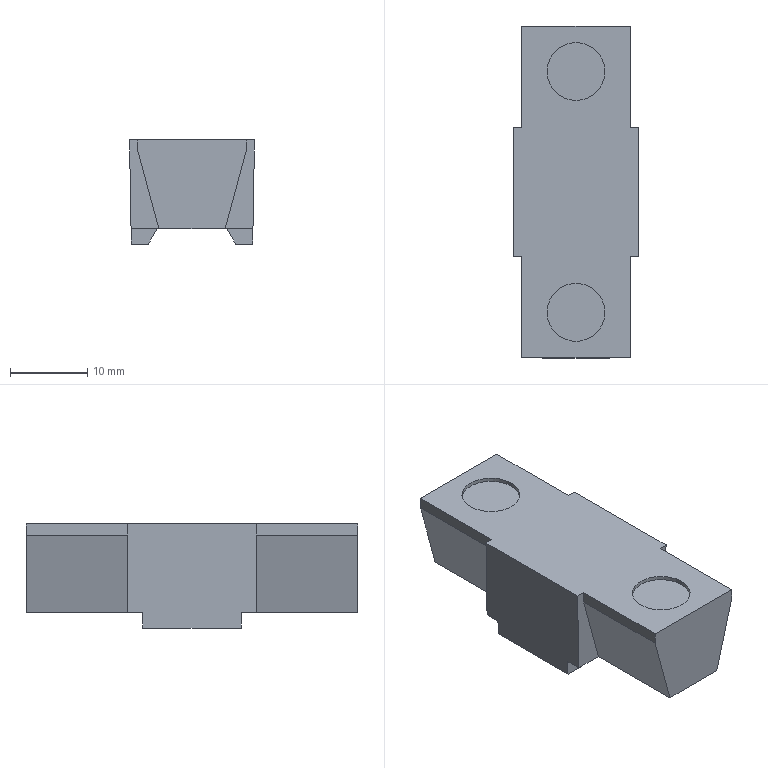Part | SolidWorks | features BaseBody 1 | 1 solid | 32 faces | box 16.2 x 43 x 13.5 mm | volume 6701 mm3 | plane 28 | cylinder 4 | commonest cylinder face diameters 7.5 x4
STEP:
#1=CARTESIAN_POINT('',(-3.75,15.6,26.));
#2=VERTEX_POINT('',#1);
#3=CARTESIAN_POINT('',(3.75,15.6,26.));
#4=VERTEX_POINT('',#3);
#5=CARTESIAN_POINT('',(0.,15.6,26.));
#6=DIRECTION('',(0.,0.,1.));
#7=DIRECTION('',(1.,0.,0.));
#8=AXIS2_PLACEMENT_3D('',#5,#6,#7);
#9=CIRCLE('',#8,3.75);
#10=EDGE_CURVE('',#2,#4,#9,.T.);
#11=ORIENTED_EDGE('',*,*,#10,.F.);
#12=CARTESIAN_POINT('',(-3.75,15.6,26.5));
#13=VERTEX_POINT('',#12);
#14=CARTESIAN_POINT('',(-3.75,15.6,26.));
#15=DIRECTION('',(0.,0.,1.));
#16=VECTOR('',#15,1000.);
#17=LINE('',#14,#16);
#18=EDGE_CURVE('',#2,#13,#17,.T.);
#19=ORIENTED_EDGE('',*,*,#18,.T.);
#20=CARTESIAN_POINT('',(3.75,15.6,26.5));
#21=VERTEX_POINT('',#20);
#22=CARTESIAN_POINT('',(0.,15.6,26.5));
#23=DIRECTION('',(0.,0.,1.));
#24=DIRECTION('',(1.,0.,0.));
#25=AXIS2_PLACEMENT_3D('',#22,#23,#24);
#26=CIRCLE('',#25,3.75);
#27=EDGE_CURVE('',#13,#21,#26,.T.);
#28=ORIENTED_EDGE('',*,*,#27,.T.);
#29=CARTESIAN_POINT('',(3.75,15.6,26.));
#30=DIRECTION('',(0.,0.,1.));
#31=VECTOR('',#30,1000.);
#32=LINE('',#29,#31);
#33=EDGE_CURVE('',#4,#21,#32,.T.);
#34=ORIENTED_EDGE('',*,*,#33,.F.);
#35=EDGE_LOOP('',(#11,#19,#28,#34));
#36=FACE_OUTER_BOUND('',#35,.T.);
#37=CARTESIAN_POINT('',(0.,15.6,26.));
#38=DIRECTION('',(0.,0.,1.));
#39=DIRECTION('',(1.,0.,0.));
#40=AXIS2_PLACEMENT_3D('',#37,#38,#39);
#41=CYLINDRICAL_SURFACE('',#40,3.75);
#42=ADVANCED_FACE('',(#36),#41,.F.);
#43=CARTESIAN_POINT('',(-3.75,-15.6,26.));
#44=VERTEX_POINT('',#43);
#45=CARTESIAN_POINT('',(3.75,-15.6,26.));
#46=VERTEX_POINT('',#45);
#47=CARTESIAN_POINT('',(0.,-15.6,26.));
#48=DIRECTION('',(0.,0.,1.));
#49=DIRECTION('',(1.,0.,0.));
#50=AXIS2_PLACEMENT_3D('',#47,#48,#49);
#51=CIRCLE('',#50,3.75);
#52=EDGE_CURVE('',#44,#46,#51,.T.);
#53=ORIENTED_EDGE('',*,*,#52,.F.);
#54=CARTESIAN_POINT('',(-3.75,-15.6,26.5));
#55=VERTEX_POINT('',#54);
#56=CARTESIAN_POINT('',(-3.75,-15.6,26.));
#57=DIRECTION('',(0.,0.,1.));
#58=VECTOR('',#57,1000.);
#59=LINE('',#56,#58);
#60=EDGE_CURVE('',#44,#55,#59,.T.);
#61=ORIENTED_EDGE('',*,*,#60,.T.);
#62=CARTESIAN_POINT('',(3.75,-15.6,26.5));
#63=VERTEX_POINT('',#62);
#64=CARTESIAN_POINT('',(0.,-15.6,26.5));
#65=DIRECTION('',(0.,0.,1.));
#66=DIRECTION('',(1.,0.,0.));
#67=AXIS2_PLACEMENT_3D('',#64,#65,#66);
#68=CIRCLE('',#67,3.75);
#69=EDGE_CURVE('',#55,#63,#68,.T.);
#70=ORIENTED_EDGE('',*,*,#69,.T.);
#71=CARTESIAN_POINT('',(3.75,-15.6,26.));
#72=DIRECTION('',(0.,0.,1.));
#73=VECTOR('',#72,1000.);
#74=LINE('',#71,#73);
#75=EDGE_CURVE('',#46,#63,#74,.T.);
#76=ORIENTED_EDGE('',*,*,#75,.F.);
#77=EDGE_LOOP('',(#53,#61,#70,#76));
#78=FACE_OUTER_BOUND('',#77,.T.);
#79=CARTESIAN_POINT('',(0.,-15.6,26.));
#80=DIRECTION('',(0.,0.,1.));
#81=DIRECTION('',(1.,0.,0.));
#82=AXIS2_PLACEMENT_3D('',#79,#80,#81);
#83=CYLINDRICAL_SURFACE('',#82,3.75);
#84=ADVANCED_FACE('',(#78),#83,.F.);
#85=CARTESIAN_POINT('',(7.864,6.4,13.));
#86=VERTEX_POINT('',#85);
#87=CARTESIAN_POINT('',(5.655,6.4,13.));
#88=VERTEX_POINT('',#87);
#89=CARTESIAN_POINT('',(7.864,6.4,13.));
#90=DIRECTION('',(-1.,0.,0.));
#91=VECTOR('',#90,1000.);
#92=LINE('',#89,#91);
#93=EDGE_CURVE('',#86,#88,#92,.T.);
#94=ORIENTED_EDGE('',*,*,#93,.F.);
#95=CARTESIAN_POINT('',(7.864,-6.4,13.));
#96=VERTEX_POINT('',#95);
#97=CARTESIAN_POINT('',(7.864,6.4,13.));
#98=DIRECTION('',(0.,-1.,0.));
#99=VECTOR('',#98,1000.);
#100=LINE('',#97,#99);
#101=EDGE_CURVE('',#86,#96,#100,.T.);
#102=ORIENTED_EDGE('',*,*,#101,.T.);
#103=CARTESIAN_POINT('',(5.655,-6.4,13.));
#104=VERTEX_POINT('',#103);
#105=CARTESIAN_POINT('',(7.864,-6.4,13.));
#106=DIRECTION('',(-1.,0.,0.));
#107=VECTOR('',#106,1000.);
#108=LINE('',#105,#107);
#109=EDGE_CURVE('',#96,#104,#108,.T.);
#110=ORIENTED_EDGE('',*,*,#109,.T.);
#111=CARTESIAN_POINT('',(5.655,6.4,13.));
#112=DIRECTION('',(0.,-1.,0.));
#113=VECTOR('',#112,1000.);
#114=LINE('',#111,#113);
#115=EDGE_CURVE('',#88,#104,#114,.T.);
#116=ORIENTED_EDGE('',*,*,#115,.F.);
#117=EDGE_LOOP('',(#94,#102,#110,#116));
#118=FACE_OUTER_BOUND('',#117,.T.);
#119=CARTESIAN_POINT('',(8.1,8.4,13.));
#120=DIRECTION('',(0.,0.,1.));
#121=DIRECTION('',(1.,0.,0.));
#122=AXIS2_PLACEMENT_3D('',#119,#120,#121);
#123=PLANE('',#122);
#124=ADVANCED_FACE('',(#118),#123,.F.);
#125=CARTESIAN_POINT('',(4.5,6.4,15.));
#126=VERTEX_POINT('',#125);
#127=CARTESIAN_POINT('',(5.655,6.4,13.));
#128=DIRECTION('',(-0.5,0.,0.866));
#129=VECTOR('',#128,1000.);
#130=LINE('',#127,#129);
#131=EDGE_CURVE('',#88,#126,#130,.T.);
#132=ORIENTED_EDGE('',*,*,#131,.T.);
#133=CARTESIAN_POINT('',(7.899,6.4,15.));
#134=VERTEX_POINT('',#133);
#135=CARTESIAN_POINT('',(7.899,6.4,15.));
#136=DIRECTION('',(-1.,0.,0.));
#137=VECTOR('',#136,1000.);
#138=LINE('',#135,#137);
#139=EDGE_CURVE('',#134,#126,#138,.T.);
#140=ORIENTED_EDGE('',*,*,#139,.F.);
#141=CARTESIAN_POINT('',(7.864,6.4,13.));
#142=DIRECTION('',(0.01745,0.,0.9998));
#143=VECTOR('',#142,1000.);
#144=LINE('',#141,#143);
#145=EDGE_CURVE('',#86,#134,#144,.T.);
#146=ORIENTED_EDGE('',*,*,#145,.F.);
#147=ORIENTED_EDGE('',*,*,#93,.T.);
#148=EDGE_LOOP('',(#132,#140,#146,#147));
#149=FACE_OUTER_BOUND('',#148,.T.);
#150=CARTESIAN_POINT('',(8.1,6.4,15.));
#151=DIRECTION('',(0.,1.,0.));
#152=DIRECTION('',(0.,0.,1.));
#153=AXIS2_PLACEMENT_3D('',#150,#151,#152);
#154=PLANE('',#153);
#155=ADVANCED_FACE('',(#149),#154,.T.);
#156=ORIENTED_EDGE('',*,*,#145,.T.);
#157=CARTESIAN_POINT('',(7.899,8.4,15.));
#158=VERTEX_POINT('',#157);
#159=CARTESIAN_POINT('',(7.899,6.4,15.));
#160=DIRECTION('',(0.,1.,0.));
#161=VECTOR('',#160,1000.);
#162=LINE('',#159,#161);
#163=EDGE_CURVE('',#134,#158,#162,.T.);
#164=ORIENTED_EDGE('',*,*,#163,.T.);
#165=CARTESIAN_POINT('',(8.1,8.4,26.5));
#166=VERTEX_POINT('',#165);
#167=CARTESIAN_POINT('',(8.1,8.4,26.5));
#168=DIRECTION('',(-0.01745,0.,-0.9998));
#169=VECTOR('',#168,1000.);
#170=LINE('',#167,#169);
#171=EDGE_CURVE('',#166,#158,#170,.T.);
#172=ORIENTED_EDGE('',*,*,#171,.F.);
#173=CARTESIAN_POINT('',(8.1,-8.4,26.5));
#174=VERTEX_POINT('',#173);
#175=CARTESIAN_POINT('',(8.1,8.4,26.5));
#176=DIRECTION('',(0.,-1.,0.));
#177=VECTOR('',#176,1000.);
#178=LINE('',#175,#177);
#179=EDGE_CURVE('',#166,#174,#178,.T.);
#180=ORIENTED_EDGE('',*,*,#179,.T.);
#181=CARTESIAN_POINT('',(7.899,-8.4,15.));
#182=VERTEX_POINT('',#181);
#183=CARTESIAN_POINT('',(8.1,-8.4,26.5));
#184=DIRECTION('',(-0.01745,0.,-0.9998));
#185=VECTOR('',#184,1000.);
#186=LINE('',#183,#185);
#187=EDGE_CURVE('',#174,#182,#186,.T.);
#188=ORIENTED_EDGE('',*,*,#187,.T.);
#189=CARTESIAN_POINT('',(7.899,-6.4,15.));
#190=VERTEX_POINT('',#189);
#191=CARTESIAN_POINT('',(7.899,-8.4,15.));
#192=DIRECTION('',(0.,1.,0.));
#193=VECTOR('',#192,1000.);
#194=LINE('',#191,#193);
#195=EDGE_CURVE('',#182,#190,#194,.T.);
#196=ORIENTED_EDGE('',*,*,#195,.T.);
#197=CARTESIAN_POINT('',(7.899,-6.4,15.));
#198=DIRECTION('',(-0.01745,0.,-0.9998));
#199=VECTOR('',#198,1000.);
#200=LINE('',#197,#199);
#201=EDGE_CURVE('',#190,#96,#200,.T.);
#202=ORIENTED_EDGE('',*,*,#201,.T.);
#203=ORIENTED_EDGE('',*,*,#101,.F.);
#204=EDGE_LOOP('',(#156,#164,#172,#180,#188,#196,#202,#203));
#205=FACE_OUTER_BOUND('',#204,.T.);
#206=CARTESIAN_POINT('',(7.864,21.5,13.));
#207=DIRECTION('',(0.9998,0.,-0.01745));
#208=DIRECTION('',(-0.01745,0.,-0.9998));
#209=AXIS2_PLACEMENT_3D('',#206,#207,#208);
#210=PLANE('',#209);
#211=ADVANCED_FACE('',(#205),#210,.T.);
#212=CARTESIAN_POINT('',(4.5,-6.4,15.));
#213=VERTEX_POINT('',#212);
#214=CARTESIAN_POINT('',(4.5,-6.4,15.));
#215=DIRECTION('',(0.5,0.,-0.866));
#216=VECTOR('',#215,1000.);
#217=LINE('',#214,#216);
#218=EDGE_CURVE('',#213,#104,#217,.T.);
#219=ORIENTED_EDGE('',*,*,#218,.T.);
#220=ORIENTED_EDGE('',*,*,#109,.F.);
#221=ORIENTED_EDGE('',*,*,#201,.F.);
#222=CARTESIAN_POINT('',(7.899,-6.4,15.));
#223=DIRECTION('',(-1.,0.,0.));
#224=VECTOR('',#223,1000.);
#225=LINE('',#222,#224);
#226=EDGE_CURVE('',#190,#213,#225,.T.);
#227=ORIENTED_EDGE('',*,*,#226,.T.);
#228=EDGE_LOOP('',(#219,#220,#221,#227));
#229=FACE_OUTER_BOUND('',#228,.T.);
#230=CARTESIAN_POINT('',(8.1,-6.4,13.));
#231=DIRECTION('',(0.,-1.,0.));
#232=DIRECTION('',(0.,0.,-1.));
#233=AXIS2_PLACEMENT_3D('',#230,#231,#232);
#234=PLANE('',#233);
#235=ADVANCED_FACE('',(#229),#234,.T.);
#236=ORIENTED_EDGE('',*,*,#131,.F.);
#237=ORIENTED_EDGE('',*,*,#115,.T.);
#238=ORIENTED_EDGE('',*,*,#218,.F.);
#239=CARTESIAN_POINT('',(4.5,6.4,15.));
#240=DIRECTION('',(0.,-1.,0.));
#241=VECTOR('',#240,1000.);
#242=LINE('',#239,#241);
#243=EDGE_CURVE('',#126,#213,#242,.T.);
#244=ORIENTED_EDGE('',*,*,#243,.F.);
#245=EDGE_LOOP('',(#236,#237,#238,#244));
#246=FACE_OUTER_BOUND('',#245,.T.);
#247=CARTESIAN_POINT('',(5.655,8.4,13.));
#248=DIRECTION('',(0.866,0.,0.5));
#249=DIRECTION('',(0.5,0.,-0.866));
#250=AXIS2_PLACEMENT_3D('',#247,#248,#249);
#251=PLANE('',#250);
#252=ADVANCED_FACE('',(#246),#251,.F.);
#253=CARTESIAN_POINT('',(-4.3,-8.4,15.));
#254=VERTEX_POINT('',#253);
#255=CARTESIAN_POINT('',(-7.899,-8.4,15.));
#256=VERTEX_POINT('',#255);
#257=CARTESIAN_POINT('',(-4.3,-8.4,15.));
#258=DIRECTION('',(-1.,0.,0.));
#259=VECTOR('',#258,1000.);
#260=LINE('',#257,#259);
#261=EDGE_CURVE('',#254,#256,#260,.T.);
#262=ORIENTED_EDGE('',*,*,#261,.T.);
#263=CARTESIAN_POINT('',(-7.899,-6.4,15.));
#264=VERTEX_POINT('',#263);
#265=CARTESIAN_POINT('',(-7.899,-6.4,15.));
#266=DIRECTION('',(0.,-1.,0.));
#267=VECTOR('',#266,1000.);
#268=LINE('',#265,#267);
#269=EDGE_CURVE('',#264,#256,#268,.T.);
#270=ORIENTED_EDGE('',*,*,#269,.F.);
#271=CARTESIAN_POINT('',(-4.5,-6.4,15.));
#272=VERTEX_POINT('',#271);
#273=CARTESIAN_POINT('',(-4.5,-6.4,15.));
#274=DIRECTION('',(-1.,0.,0.));
#275=VECTOR('',#274,1000.);
#276=LINE('',#273,#275);
#277=EDGE_CURVE('',#272,#264,#276,.T.);
#278=ORIENTED_EDGE('',*,*,#277,.F.);
#279=CARTESIAN_POINT('',(-4.5,6.4,15.));
#280=VERTEX_POINT('',#279);
#281=CARTESIAN_POINT('',(-4.5,6.4,15.));
#282=DIRECTION('',(0.,-1.,0.));
#283=VECTOR('',#282,1000.);
#284=LINE('',#281,#283);
#285=EDGE_CURVE('',#280,#272,#284,.T.);
#286=ORIENTED_EDGE('',*,*,#285,.F.);
#287=CARTESIAN_POINT('',(-7.899,6.4,15.));
#288=VERTEX_POINT('',#287);
#289=CARTESIAN_POINT('',(-4.5,6.4,15.));
#290=DIRECTION('',(-1.,0.,0.));
#291=VECTOR('',#290,1000.);
#292=LINE('',#289,#291);
#293=EDGE_CURVE('',#280,#288,#292,.T.);
#294=ORIENTED_EDGE('',*,*,#293,.T.);
#295=CARTESIAN_POINT('',(-7.899,8.4,15.));
#296=VERTEX_POINT('',#295);
#297=CARTESIAN_POINT('',(-7.899,8.4,15.));
#298=DIRECTION('',(0.,-1.,0.));
#299=VECTOR('',#298,1000.);
#300=LINE('',#297,#299);
#301=EDGE_CURVE('',#296,#288,#300,.T.);
#302=ORIENTED_EDGE('',*,*,#301,.F.);
#303=CARTESIAN_POINT('',(-4.3,8.4,15.));
#304=VERTEX_POINT('',#303);
#305=CARTESIAN_POINT('',(-4.3,8.4,15.));
#306=DIRECTION('',(-1.,0.,0.));
#307=VECTOR('',#306,1000.);
#308=LINE('',#305,#307);
#309=EDGE_CURVE('',#304,#296,#308,.T.);
#310=ORIENTED_EDGE('',*,*,#309,.F.);
#311=CARTESIAN_POINT('',(-4.3,21.5,15.));
#312=VERTEX_POINT('',#311);
#313=CARTESIAN_POINT('',(-4.3,21.5,15.));
#314=DIRECTION('',(0.,-1.,0.));
#315=VECTOR('',#314,1000.);
#316=LINE('',#313,#315);
#317=EDGE_CURVE('',#312,#304,#316,.T.);
#318=ORIENTED_EDGE('',*,*,#317,.F.);
#319=CARTESIAN_POINT('',(4.3,21.5,15.));
#320=VERTEX_POINT('',#319);
#321=CARTESIAN_POINT('',(4.3,21.5,15.));
#322=DIRECTION('',(-1.,0.,0.));
#323=VECTOR('',#322,1000.);
#324=LINE('',#321,#323);
#325=EDGE_CURVE('',#320,#312,#324,.T.);
#326=ORIENTED_EDGE('',*,*,#325,.F.);
#327=CARTESIAN_POINT('',(4.3,8.4,15.));
#328=VERTEX_POINT('',#327);
#329=CARTESIAN_POINT('',(4.3,21.5,15.));
#330=DIRECTION('',(0.,-1.,0.));
#331=VECTOR('',#330,1000.);
#332=LINE('',#329,#331);
#333=EDGE_CURVE('',#320,#328,#332,.T.);
#334=ORIENTED_EDGE('',*,*,#333,.T.);
#335=CARTESIAN_POINT('',(7.899,8.4,15.));
#336=DIRECTION('',(-1.,0.,0.));
#337=VECTOR('',#336,1000.);
#338=LINE('',#335,#337);
#339=EDGE_CURVE('',#158,#328,#338,.T.);
#340=ORIENTED_EDGE('',*,*,#339,.F.);
#341=ORIENTED_EDGE('',*,*,#163,.F.);
#342=ORIENTED_EDGE('',*,*,#139,.T.);
#343=ORIENTED_EDGE('',*,*,#243,.T.);
#344=ORIENTED_EDGE('',*,*,#226,.F.);
#345=ORIENTED_EDGE('',*,*,#195,.F.);
#346=CARTESIAN_POINT('',(4.3,-8.4,15.));
#347=VERTEX_POINT('',#346);
#348=CARTESIAN_POINT('',(7.899,-8.4,15.));
#349=DIRECTION('',(-1.,0.,0.));
#350=VECTOR('',#349,1000.);
#351=LINE('',#348,#350);
#352=EDGE_CURVE('',#182,#347,#351,.T.);
#353=ORIENTED_EDGE('',*,*,#352,.T.);
#354=CARTESIAN_POINT('',(4.3,-21.5,15.));
#355=VERTEX_POINT('',#354);
#356=CARTESIAN_POINT('',(4.3,-8.4,15.));
#357=DIRECTION('',(0.,-1.,0.));
#358=VECTOR('',#357,1000.);
#359=LINE('',#356,#358);
#360=EDGE_CURVE('',#347,#355,#359,.T.);
#361=ORIENTED_EDGE('',*,*,#360,.T.);
#362=CARTESIAN_POINT('',(-4.3,-21.5,15.));
#363=VERTEX_POINT('',#362);
#364=CARTESIAN_POINT('',(4.3,-21.5,15.));
#365=DIRECTION('',(-1.,0.,0.));
#366=VECTOR('',#365,1000.);
#367=LINE('',#364,#366);
#368=EDGE_CURVE('',#355,#363,#367,.T.);
#369=ORIENTED_EDGE('',*,*,#368,.T.);
#370=CARTESIAN_POINT('',(-4.3,-8.4,15.));
#371=DIRECTION('',(0.,-1.,0.));
#372=VECTOR('',#371,1000.);
#373=LINE('',#370,#372);
#374=EDGE_CURVE('',#254,#363,#373,.T.);
#375=ORIENTED_EDGE('',*,*,#374,.F.);
#376=EDGE_LOOP('',(#262,#270,#278,#286,#294,#302,#310,#318,#326,#334,#340,#341,#342,#343,#344,#345,#353,#361,#369,#375));
#377=FACE_OUTER_BOUND('',#376,.T.);
#378=CARTESIAN_POINT('',(4.3,21.5,15.));
#379=DIRECTION('',(0.,0.,1.));
#380=DIRECTION('',(1.,0.,0.));
#381=AXIS2_PLACEMENT_3D('',#378,#379,#380);
#382=PLANE('',#381);
#383=ADVANCED_FACE('',(#377),#382,.F.);
#384=ORIENTED_EDGE('',*,*,#171,.T.);
#385=ORIENTED_EDGE('',*,*,#339,.T.);
#386=CARTESIAN_POINT('',(7.,8.4,25.));
#387=VERTEX_POINT('',#386);
#388=CARTESIAN_POINT('',(7.,8.4,25.));
#389=DIRECTION('',(-0.2607,0.,-0.9654));
#390=VECTOR('',#389,1000.);
#391=LINE('',#388,#390);
#392=EDGE_CURVE('',#387,#328,#391,.T.);
#393=ORIENTED_EDGE('',*,*,#392,.F.);
#394=CARTESIAN_POINT('',(7.,8.4,26.5));
#395=VERTEX_POINT('',#394);
#396=CARTESIAN_POINT('',(7.,8.4,26.5));
#397=DIRECTION('',(0.,0.,-1.));
#398=VECTOR('',#397,1000.);
#399=LINE('',#396,#398);
#400=EDGE_CURVE('',#395,#387,#399,.T.);
#401=ORIENTED_EDGE('',*,*,#400,.F.);
#402=CARTESIAN_POINT('',(7.,8.4,26.5));
#403=DIRECTION('',(1.,0.,0.));
#404=VECTOR('',#403,1000.);
#405=LINE('',#402,#404);
#406=EDGE_CURVE('',#395,#166,#405,.T.);
#407=ORIENTED_EDGE('',*,*,#406,.T.);
#408=EDGE_LOOP('',(#384,#385,#393,#401,#407));
#409=FACE_OUTER_BOUND('',#408,.T.);
#410=CARTESIAN_POINT('',(0.,8.4,0.));
#411=DIRECTION('',(0.,1.,0.));
#412=DIRECTION('',(0.,0.,1.));
#413=AXIS2_PLACEMENT_3D('',#410,#411,#412);
#414=PLANE('',#413);
#415=ADVANCED_FACE('',(#409),#414,.T.);
#416=CARTESIAN_POINT('',(0.,-15.6,26.5));
#417=DIRECTION('',(0.,0.,1.));
#418=DIRECTION('',(1.,0.,0.));
#419=AXIS2_PLACEMENT_3D('',#416,#417,#418);
#420=CIRCLE('',#419,3.75);
#421=EDGE_CURVE('',#63,#55,#420,.T.);
#422=ORIENTED_EDGE('',*,*,#421,.F.);
#423=ORIENTED_EDGE('',*,*,#69,.F.);
#424=EDGE_LOOP('',(#422,#423));
#425=FACE_BOUND('',#424,.T.);
#426=CARTESIAN_POINT('',(0.,15.6,26.5));
#427=DIRECTION('',(0.,0.,1.));
#428=DIRECTION('',(1.,0.,0.));
#429=AXIS2_PLACEMENT_3D('',#426,#427,#428);
#430=CIRCLE('',#429,3.75);
#431=EDGE_CURVE('',#21,#13,#430,.T.);
#432=ORIENTED_EDGE('',*,*,#431,.F.);
#433=ORIENTED_EDGE('',*,*,#27,.F.);
#434=EDGE_LOOP('',(#432,#433));
#435=FACE_BOUND('',#434,.T.);
#436=CARTESIAN_POINT('',(-7.,21.5,26.5));
#437=VERTEX_POINT('',#436);
#438=CARTESIAN_POINT('',(-7.,8.4,26.5));
#439=VERTEX_POINT('',#438);
#440=CARTESIAN_POINT('',(-7.,21.5,26.5));
#441=DIRECTION('',(0.,-1.,0.));
#442=VECTOR('',#441,1000.);
#443=LINE('',#440,#442);
#444=EDGE_CURVE('',#437,#439,#443,.T.);
#445=ORIENTED_EDGE('',*,*,#444,.T.);
#446=CARTESIAN_POINT('',(-8.1,8.4,26.5));
#447=VERTEX_POINT('',#446);
#448=CARTESIAN_POINT('',(-8.1,8.4,26.5));
#449=DIRECTION('',(1.,0.,0.));
#450=VECTOR('',#449,1000.);
#451=LINE('',#448,#450);
#452=EDGE_CURVE('',#447,#439,#451,.T.);
#453=ORIENTED_EDGE('',*,*,#452,.F.);
#454=CARTESIAN_POINT('',(-8.1,-8.4,26.5));
#455=VERTEX_POINT('',#454);
#456=CARTESIAN_POINT('',(-8.1,8.4,26.5));
#457=DIRECTION('',(0.,-1.,0.));
#458=VECTOR('',#457,1000.);
#459=LINE('',#456,#458);
#460=EDGE_CURVE('',#447,#455,#459,.T.);
#461=ORIENTED_EDGE('',*,*,#460,.T.);
#462=CARTESIAN_POINT('',(-7.,-8.4,26.5));
#463=VERTEX_POINT('',#462);
#464=CARTESIAN_POINT('',(-8.1,-8.4,26.5));
#465=DIRECTION('',(1.,0.,0.));
#466=VECTOR('',#465,1000.);
#467=LINE('',#464,#466);
#468=EDGE_CURVE('',#455,#463,#467,.T.);
#469=ORIENTED_EDGE('',*,*,#468,.T.);
#470=CARTESIAN_POINT('',(-7.,-21.5,26.5));
#471=VERTEX_POINT('',#470);
#472=CARTESIAN_POINT('',(-7.,-8.4,26.5));
#473=DIRECTION('',(0.,-1.,0.));
#474=VECTOR('',#473,1000.);
#475=LINE('',#472,#474);
#476=EDGE_CURVE('',#463,#471,#475,.T.);
#477=ORIENTED_EDGE('',*,*,#476,.T.);
#478=CARTESIAN_POINT('',(7.,-21.5,26.5));
#479=VERTEX_POINT('',#478);
#480=CARTESIAN_POINT('',(-7.,-21.5,26.5));
#481=DIRECTION('',(1.,0.,0.));
#482=VECTOR('',#481,1000.);
#483=LINE('',#480,#482);
#484=EDGE_CURVE('',#471,#479,#483,.T.);
#485=ORIENTED_EDGE('',*,*,#484,.T.);
#486=CARTESIAN_POINT('',(7.,-8.4,26.5));
#487=VERTEX_POINT('',#486);
#488=CARTESIAN_POINT('',(7.,-8.4,26.5));
#489=DIRECTION('',(0.,-1.,0.));
#490=VECTOR('',#489,1000.);
#491=LINE('',#488,#490);
#492=EDGE_CURVE('',#487,#479,#491,.T.);
#493=ORIENTED_EDGE('',*,*,#492,.F.);
#494=CARTESIAN_POINT('',(7.,-8.4,26.5));
#495=DIRECTION('',(1.,0.,0.));
#496=VECTOR('',#495,1000.);
#497=LINE('',#494,#496);
#498=EDGE_CURVE('',#487,#174,#497,.T.);
#499=ORIENTED_EDGE('',*,*,#498,.T.);
#500=ORIENTED_EDGE('',*,*,#179,.F.);
#501=ORIENTED_EDGE('',*,*,#406,.F.);
#502=CARTESIAN_POINT('',(7.,21.5,26.5));
#503=VERTEX_POINT('',#502);
#504=CARTESIAN_POINT('',(7.,21.5,26.5));
#505=DIRECTION('',(0.,-1.,0.));
#506=VECTOR('',#505,1000.);
#507=LINE('',#504,#506);
#508=EDGE_CURVE('',#503,#395,#507,.T.);
#509=ORIENTED_EDGE('',*,*,#508,.F.);
#510=CARTESIAN_POINT('',(-7.,21.5,26.5));
#511=DIRECTION('',(1.,0.,0.));
#512=VECTOR('',#511,1000.);
#513=LINE('',#510,#512);
#514=EDGE_CURVE('',#437,#503,#513,.T.);
#515=ORIENTED_EDGE('',*,*,#514,.F.);
#516=EDGE_LOOP('',(#445,#453,#461,#469,#477,#485,#493,#499,#500,#501,#509,#515));
#517=FACE_OUTER_BOUND('',#516,.T.);
#518=CARTESIAN_POINT('',(-7.,21.5,26.5));
#519=DIRECTION('',(0.,0.,-1.));
#520=DIRECTION('',(-1.,0.,0.));
#521=AXIS2_PLACEMENT_3D('',#518,#519,#520);
#522=PLANE('',#521);
#523=ADVANCED_FACE('',(#425,#435,#517),#522,.F.);
#524=ORIENTED_EDGE('',*,*,#352,.F.);
#525=ORIENTED_EDGE('',*,*,#187,.F.);
#526=ORIENTED_EDGE('',*,*,#498,.F.);
#527=CARTESIAN_POINT('',(7.,-8.4,25.));
#528=VERTEX_POINT('',#527);
#529=CARTESIAN_POINT('',(7.,-8.4,26.5));
#530=DIRECTION('',(0.,0.,-1.));
#531=VECTOR('',#530,1000.);
#532=LINE('',#529,#531);
#533=EDGE_CURVE('',#487,#528,#532,.T.);
#534=ORIENTED_EDGE('',*,*,#533,.T.);
#535=CARTESIAN_POINT('',(7.,-8.4,25.));
#536=DIRECTION('',(-0.2607,0.,-0.9654));
#537=VECTOR('',#536,1000.);
#538=LINE('',#535,#537);
#539=EDGE_CURVE('',#528,#347,#538,.T.);
#540=ORIENTED_EDGE('',*,*,#539,.T.);
#541=EDGE_LOOP('',(#524,#525,#526,#534,#540));
#542=FACE_OUTER_BOUND('',#541,.T.);
#543=CARTESIAN_POINT('',(0.,-8.4,0.));
#544=DIRECTION('',(0.,1.,0.));
#545=DIRECTION('',(0.,0.,1.));
#546=AXIS2_PLACEMENT_3D('',#543,#544,#545);
#547=PLANE('',#546);
#548=ADVANCED_FACE('',(#542),#547,.F.);
#549=CARTESIAN_POINT('',(-7.899,-8.4,15.));
#550=DIRECTION('',(-0.01745,0.,0.9998));
#551=VECTOR('',#550,1000.);
#552=LINE('',#549,#551);
#553=EDGE_CURVE('',#256,#455,#552,.T.);
#554=ORIENTED_EDGE('',*,*,#553,.F.);
#555=ORIENTED_EDGE('',*,*,#261,.F.);
#556=CARTESIAN_POINT('',(-7.,-8.4,25.));
#557=VERTEX_POINT('',#556);
#558=CARTESIAN_POINT('',(-4.3,-8.4,15.));
#559=DIRECTION('',(-0.2607,0.,0.9654));
#560=VECTOR('',#559,1000.);
#561=LINE('',#558,#560);
#562=EDGE_CURVE('',#254,#557,#561,.T.);
#563=ORIENTED_EDGE('',*,*,#562,.T.);
#564=CARTESIAN_POINT('',(-7.,-8.4,25.));
#565=DIRECTION('',(0.,0.,1.));
#566=VECTOR('',#565,1000.);
#567=LINE('',#564,#566);
#568=EDGE_CURVE('',#557,#463,#567,.T.);
#569=ORIENTED_EDGE('',*,*,#568,.T.);
#570=ORIENTED_EDGE('',*,*,#468,.F.);
#571=EDGE_LOOP('',(#554,#555,#563,#569,#570));
#572=FACE_OUTER_BOUND('',#571,.T.);
#573=CARTESIAN_POINT('',(0.,-8.4,0.));
#574=DIRECTION('',(0.,1.,0.));
#575=DIRECTION('',(0.,0.,1.));
#576=AXIS2_PLACEMENT_3D('',#573,#574,#575);
#577=PLANE('',#576);
#578=ADVANCED_FACE('',(#572),#577,.F.);
#579=CARTESIAN_POINT('',(-7.899,8.4,15.));
#580=DIRECTION('',(-0.01745,0.,0.9998));
#581=VECTOR('',#580,1000.);
#582=LINE('',#579,#581);
#583=EDGE_CURVE('',#296,#447,#582,.T.);
#584=ORIENTED_EDGE('',*,*,#583,.F.);
#585=ORIENTED_EDGE('',*,*,#301,.T.);
#586=CARTESIAN_POINT('',(-7.864,6.4,13.));
#587=VERTEX_POINT('',#586);
#588=CARTESIAN_POINT('',(-7.899,6.4,15.));
#589=DIRECTION('',(0.01745,0.,-0.9998));
#590=VECTOR('',#589,1000.);
#591=LINE('',#588,#590);
#592=EDGE_CURVE('',#288,#587,#591,.T.);
#593=ORIENTED_EDGE('',*,*,#592,.T.);
#594=CARTESIAN_POINT('',(-7.864,-6.4,13.));
#595=VERTEX_POINT('',#594);
#596=CARTESIAN_POINT('',(-7.864,6.4,13.));
#597=DIRECTION('',(0.,-1.,0.));
#598=VECTOR('',#597,1000.);
#599=LINE('',#596,#598);
#600=EDGE_CURVE('',#587,#595,#599,.T.);
#601=ORIENTED_EDGE('',*,*,#600,.T.);
#602=CARTESIAN_POINT('',(-7.864,-6.4,13.));
#603=DIRECTION('',(-0.01745,0.,0.9998));
#604=VECTOR('',#603,1000.);
#605=LINE('',#602,#604);
#606=EDGE_CURVE('',#595,#264,#605,.T.);
#607=ORIENTED_EDGE('',*,*,#606,.T.);
#608=ORIENTED_EDGE('',*,*,#269,.T.);
#609=ORIENTED_EDGE('',*,*,#553,.T.);
#610=ORIENTED_EDGE('',*,*,#460,.F.);
#611=EDGE_LOOP('',(#584,#585,#593,#601,#607,#608,#609,#610));
#612=FACE_OUTER_BOUND('',#611,.T.);
#613=CARTESIAN_POINT('',(-8.1,21.5,26.5));
#614=DIRECTION('',(-0.9998,0.,-0.01745));
#615=DIRECTION('',(-0.01745,0.,0.9998));
#616=AXIS2_PLACEMENT_3D('',#613,#614,#615);
#617=PLANE('',#616);
#618=ADVANCED_FACE('',(#612),#617,.T.);
#619=CARTESIAN_POINT('',(-5.655,-6.4,13.));
#620=VERTEX_POINT('',#619);
#621=CARTESIAN_POINT('',(-5.655,-6.4,13.));
#622=DIRECTION('',(0.5,0.,0.866));
#623=VECTOR('',#622,1000.);
#624=LINE('',#621,#623);
#625=EDGE_CURVE('',#620,#272,#624,.T.);
#626=ORIENTED_EDGE('',*,*,#625,.T.);
#627=ORIENTED_EDGE('',*,*,#277,.T.);
#628=ORIENTED_EDGE('',*,*,#606,.F.);
#629=CARTESIAN_POINT('',(-5.655,-6.4,13.));
#630=DIRECTION('',(-1.,0.,0.));
#631=VECTOR('',#630,1000.);
#632=LINE('',#629,#631);
#633=EDGE_CURVE('',#620,#595,#632,.T.);
#634=ORIENTED_EDGE('',*,*,#633,.F.);
#635=EDGE_LOOP('',(#626,#627,#628,#634));
#636=FACE_OUTER_BOUND('',#635,.T.);
#637=CARTESIAN_POINT('',(8.1,-6.4,13.));
#638=DIRECTION('',(0.,-1.,0.));
#639=DIRECTION('',(0.,0.,-1.));
#640=AXIS2_PLACEMENT_3D('',#637,#638,#639);
#641=PLANE('',#640);
#642=ADVANCED_FACE('',(#636),#641,.T.);
#643=CARTESIAN_POINT('',(-5.655,6.4,13.));
#644=VERTEX_POINT('',#643);
#645=CARTESIAN_POINT('',(-4.5,6.4,15.));
#646=DIRECTION('',(-0.5,0.,-0.866));
#647=VECTOR('',#646,1000.);
#648=LINE('',#645,#647);
#649=EDGE_CURVE('',#280,#644,#648,.T.);
#650=ORIENTED_EDGE('',*,*,#649,.F.);
#651=ORIENTED_EDGE('',*,*,#285,.T.);
#652=ORIENTED_EDGE('',*,*,#625,.F.);
#653=CARTESIAN_POINT('',(-5.655,6.4,13.));
#654=DIRECTION('',(0.,-1.,0.));
#655=VECTOR('',#654,1000.);
#656=LINE('',#653,#655);
#657=EDGE_CURVE('',#644,#620,#656,.T.);
#658=ORIENTED_EDGE('',*,*,#657,.F.);
#659=EDGE_LOOP('',(#650,#651,#652,#658));
#660=FACE_OUTER_BOUND('',#659,.T.);
#661=CARTESIAN_POINT('',(-4.5,8.4,15.));
#662=DIRECTION('',(-0.866,0.,0.5));
#663=DIRECTION('',(0.5,0.,0.866));
#664=AXIS2_PLACEMENT_3D('',#661,#662,#663);
#665=PLANE('',#664);
#666=ADVANCED_FACE('',(#660),#665,.F.);
#667=ORIENTED_EDGE('',*,*,#649,.T.);
#668=CARTESIAN_POINT('',(-5.655,6.4,13.));
#669=DIRECTION('',(-1.,0.,0.));
#670=VECTOR('',#669,1000.);
#671=LINE('',#668,#670);
#672=EDGE_CURVE('',#644,#587,#671,.T.);
#673=ORIENTED_EDGE('',*,*,#672,.T.);
#674=ORIENTED_EDGE('',*,*,#592,.F.);
#675=ORIENTED_EDGE('',*,*,#293,.F.);
#676=EDGE_LOOP('',(#667,#673,#674,#675));
#677=FACE_OUTER_BOUND('',#676,.T.);
#678=CARTESIAN_POINT('',(8.1,6.4,15.));
#679=DIRECTION('',(0.,1.,0.));
#680=DIRECTION('',(0.,0.,1.));
#681=AXIS2_PLACEMENT_3D('',#678,#679,#680);
#682=PLANE('',#681);
#683=ADVANCED_FACE('',(#677),#682,.T.);
#684=ORIENTED_EDGE('',*,*,#309,.T.);
#685=ORIENTED_EDGE('',*,*,#583,.T.);
#686=ORIENTED_EDGE('',*,*,#452,.T.);
#687=CARTESIAN_POINT('',(-7.,8.4,25.));
#688=VERTEX_POINT('',#687);
#689=CARTESIAN_POINT('',(-7.,8.4,25.));
#690=DIRECTION('',(0.,0.,1.));
#691=VECTOR('',#690,1000.);
#692=LINE('',#689,#691);
#693=EDGE_CURVE('',#688,#439,#692,.T.);
#694=ORIENTED_EDGE('',*,*,#693,.F.);
#695=CARTESIAN_POINT('',(-4.3,8.4,15.));
#696=DIRECTION('',(-0.2607,0.,0.9654));
#697=VECTOR('',#696,1000.);
#698=LINE('',#695,#697);
#699=EDGE_CURVE('',#304,#688,#698,.T.);
#700=ORIENTED_EDGE('',*,*,#699,.F.);
#701=EDGE_LOOP('',(#684,#685,#686,#694,#700));
#702=FACE_OUTER_BOUND('',#701,.T.);
#703=CARTESIAN_POINT('',(0.,8.4,0.));
#704=DIRECTION('',(0.,1.,0.));
#705=DIRECTION('',(0.,0.,1.));
#706=AXIS2_PLACEMENT_3D('',#703,#704,#705);
#707=PLANE('',#706);
#708=ADVANCED_FACE('',(#702),#707,.T.);
#709=ORIENTED_EDGE('',*,*,#317,.T.);
#710=ORIENTED_EDGE('',*,*,#699,.T.);
#711=CARTESIAN_POINT('',(-7.,21.5,25.));
#712=VERTEX_POINT('',#711);
#713=CARTESIAN_POINT('',(-7.,21.5,25.));
#714=DIRECTION('',(0.,-1.,0.));
#715=VECTOR('',#714,1000.);
#716=LINE('',#713,#715);
#717=EDGE_CURVE('',#712,#688,#716,.T.);
#718=ORIENTED_EDGE('',*,*,#717,.F.);
#719=CARTESIAN_POINT('',(-4.3,21.5,15.));
#720=DIRECTION('',(-0.2607,0.,0.9654));
#721=VECTOR('',#720,1000.);
#722=LINE('',#719,#721);
#723=EDGE_CURVE('',#312,#712,#722,.T.);
#724=ORIENTED_EDGE('',*,*,#723,.F.);
#725=EDGE_LOOP('',(#709,#710,#718,#724));
#726=FACE_OUTER_BOUND('',#725,.T.);
#727=CARTESIAN_POINT('',(-4.3,21.5,15.));
#728=DIRECTION('',(0.9654,0.,0.2607));
#729=DIRECTION('',(0.2607,0.,-0.9654));
#730=AXIS2_PLACEMENT_3D('',#727,#728,#729);
#731=PLANE('',#730);
#732=ADVANCED_FACE('',(#726),#731,.F.);
#733=ORIENTED_EDGE('',*,*,#723,.T.);
#734=CARTESIAN_POINT('',(-7.,21.5,25.));
#735=DIRECTION('',(0.,0.,1.));
#736=VECTOR('',#735,1000.);
#737=LINE('',#734,#736);
#738=EDGE_CURVE('',#712,#437,#737,.T.);
#739=ORIENTED_EDGE('',*,*,#738,.T.);
#740=ORIENTED_EDGE('',*,*,#514,.T.);
#741=CARTESIAN_POINT('',(7.,21.5,25.));
#742=VERTEX_POINT('',#741);
#743=CARTESIAN_POINT('',(7.,21.5,26.5));
#744=DIRECTION('',(0.,0.,-1.));
#745=VECTOR('',#744,1000.);
#746=LINE('',#743,#745);
#747=EDGE_CURVE('',#503,#742,#746,.T.);
#748=ORIENTED_EDGE('',*,*,#747,.T.);
#749=CARTESIAN_POINT('',(7.,21.5,25.));
#750=DIRECTION('',(-0.2607,0.,-0.9654));
#751=VECTOR('',#750,1000.);
#752=LINE('',#749,#751);
#753=EDGE_CURVE('',#742,#320,#752,.T.);
#754=ORIENTED_EDGE('',*,*,#753,.T.);
#755=ORIENTED_EDGE('',*,*,#325,.T.);
#756=EDGE_LOOP('',(#733,#739,#740,#748,#754,#755));
#757=FACE_OUTER_BOUND('',#756,.T.);
#758=CARTESIAN_POINT('',(0.,21.5,0.));
#759=DIRECTION('',(0.,1.,0.));
#760=DIRECTION('',(0.,0.,1.));
#761=AXIS2_PLACEMENT_3D('',#758,#759,#760);
#762=PLANE('',#761);
#763=ADVANCED_FACE('',(#757),#762,.T.);
#764=CARTESIAN_POINT('',(7.,21.5,25.));
#765=DIRECTION('',(0.,-1.,0.));
#766=VECTOR('',#765,1000.);
#767=LINE('',#764,#766);
#768=EDGE_CURVE('',#742,#387,#767,.T.);
#769=ORIENTED_EDGE('',*,*,#768,.T.);
#770=ORIENTED_EDGE('',*,*,#392,.T.);
#771=ORIENTED_EDGE('',*,*,#333,.F.);
#772=ORIENTED_EDGE('',*,*,#753,.F.);
#773=EDGE_LOOP('',(#769,#770,#771,#772));
#774=FACE_OUTER_BOUND('',#773,.T.);
#775=CARTESIAN_POINT('',(7.,21.5,25.));
#776=DIRECTION('',(-0.9654,0.,0.2607));
#777=DIRECTION('',(0.2607,0.,0.9654));
#778=AXIS2_PLACEMENT_3D('',#775,#776,#777);
#779=PLANE('',#778);
#780=ADVANCED_FACE('',(#774),#779,.F.);
#781=ORIENTED_EDGE('',*,*,#539,.F.);
#782=CARTESIAN_POINT('',(7.,-21.5,25.));
#783=VERTEX_POINT('',#782);
#784=CARTESIAN_POINT('',(7.,-8.4,25.));
#785=DIRECTION('',(0.,-1.,0.));
#786=VECTOR('',#785,1000.);
#787=LINE('',#784,#786);
#788=EDGE_CURVE('',#528,#783,#787,.T.);
#789=ORIENTED_EDGE('',*,*,#788,.T.);
#790=CARTESIAN_POINT('',(7.,-21.5,25.));
#791=DIRECTION('',(-0.2607,0.,-0.9654));
#792=VECTOR('',#791,1000.);
#793=LINE('',#790,#792);
#794=EDGE_CURVE('',#783,#355,#793,.T.);
#795=ORIENTED_EDGE('',*,*,#794,.T.);
#796=ORIENTED_EDGE('',*,*,#360,.F.);
#797=EDGE_LOOP('',(#781,#789,#795,#796));
#798=FACE_OUTER_BOUND('',#797,.T.);
#799=CARTESIAN_POINT('',(7.,21.5,25.));
#800=DIRECTION('',(-0.9654,0.,0.2607));
#801=DIRECTION('',(0.2607,0.,0.9654));
#802=AXIS2_PLACEMENT_3D('',#799,#800,#801);
#803=PLANE('',#802);
#804=ADVANCED_FACE('',(#798),#803,.F.);
#805=CARTESIAN_POINT('',(-7.,-21.5,25.));
#806=VERTEX_POINT('',#805);
#807=CARTESIAN_POINT('',(-4.3,-21.5,15.));
#808=DIRECTION('',(-0.2607,0.,0.9654));
#809=VECTOR('',#808,1000.);
#810=LINE('',#807,#809);
#811=EDGE_CURVE('',#363,#806,#810,.T.);
#812=ORIENTED_EDGE('',*,*,#811,.F.);
#813=ORIENTED_EDGE('',*,*,#368,.F.);
#814=ORIENTED_EDGE('',*,*,#794,.F.);
#815=CARTESIAN_POINT('',(7.,-21.5,26.5));
#816=DIRECTION('',(0.,0.,-1.));
#817=VECTOR('',#816,1000.);
#818=LINE('',#815,#817);
#819=EDGE_CURVE('',#479,#783,#818,.T.);
#820=ORIENTED_EDGE('',*,*,#819,.F.);
#821=ORIENTED_EDGE('',*,*,#484,.F.);
#822=CARTESIAN_POINT('',(-7.,-21.5,25.));
#823=DIRECTION('',(0.,0.,1.));
#824=VECTOR('',#823,1000.);
#825=LINE('',#822,#824);
#826=EDGE_CURVE('',#806,#471,#825,.T.);
#827=ORIENTED_EDGE('',*,*,#826,.F.);
#828=EDGE_LOOP('',(#812,#813,#814,#820,#821,#827));
#829=FACE_OUTER_BOUND('',#828,.T.);
#830=CARTESIAN_POINT('',(0.,-21.5,0.));
#831=DIRECTION('',(0.,1.,0.));
#832=DIRECTION('',(0.,0.,1.));
#833=AXIS2_PLACEMENT_3D('',#830,#831,#832);
#834=PLANE('',#833);
#835=ADVANCED_FACE('',(#829),#834,.F.);
#836=ORIENTED_EDGE('',*,*,#562,.F.);
#837=ORIENTED_EDGE('',*,*,#374,.T.);
#838=ORIENTED_EDGE('',*,*,#811,.T.);
#839=CARTESIAN_POINT('',(-7.,-8.4,25.));
#840=DIRECTION('',(0.,-1.,0.));
#841=VECTOR('',#840,1000.);
#842=LINE('',#839,#841);
#843=EDGE_CURVE('',#557,#806,#842,.T.);
#844=ORIENTED_EDGE('',*,*,#843,.F.);
#845=EDGE_LOOP('',(#836,#837,#838,#844));
#846=FACE_OUTER_BOUND('',#845,.T.);
#847=CARTESIAN_POINT('',(-4.3,21.5,15.));
#848=DIRECTION('',(0.9654,0.,0.2607));
#849=DIRECTION('',(0.2607,0.,-0.9654));
#850=AXIS2_PLACEMENT_3D('',#847,#848,#849);
#851=PLANE('',#850);
#852=ADVANCED_FACE('',(#846),#851,.F.);
#853=ORIENTED_EDGE('',*,*,#508,.T.);
#854=ORIENTED_EDGE('',*,*,#400,.T.);
#855=ORIENTED_EDGE('',*,*,#768,.F.);
#856=ORIENTED_EDGE('',*,*,#747,.F.);
#857=EDGE_LOOP('',(#853,#854,#855,#856));
#858=FACE_OUTER_BOUND('',#857,.T.);
#859=CARTESIAN_POINT('',(7.,21.5,26.5));
#860=DIRECTION('',(-1.,0.,0.));
#861=DIRECTION('',(0.,0.,1.));
#862=AXIS2_PLACEMENT_3D('',#859,#860,#861);
#863=PLANE('',#862);
#864=ADVANCED_FACE('',(#858),#863,.F.);
#865=ORIENTED_EDGE('',*,*,#60,.F.);
#866=CARTESIAN_POINT('',(0.,-15.6,26.));
#867=DIRECTION('',(0.,0.,1.));
#868=DIRECTION('',(1.,0.,0.));
#869=AXIS2_PLACEMENT_3D('',#866,#867,#868);
#870=CIRCLE('',#869,3.75);
#871=EDGE_CURVE('',#46,#44,#870,.T.);
#872=ORIENTED_EDGE('',*,*,#871,.F.);
#873=ORIENTED_EDGE('',*,*,#75,.T.);
#874=ORIENTED_EDGE('',*,*,#421,.T.);
#875=EDGE_LOOP('',(#865,#872,#873,#874));
#876=FACE_OUTER_BOUND('',#875,.T.);
#877=CARTESIAN_POINT('',(0.,-15.6,26.));
#878=DIRECTION('',(0.,0.,1.));
#879=DIRECTION('',(1.,0.,0.));
#880=AXIS2_PLACEMENT_3D('',#877,#878,#879);
#881=CYLINDRICAL_SURFACE('',#880,3.75);
#882=ADVANCED_FACE('',(#876),#881,.F.);
#883=ORIENTED_EDGE('',*,*,#18,.F.);
#884=CARTESIAN_POINT('',(0.,15.6,26.));
#885=DIRECTION('',(0.,0.,1.));
#886=DIRECTION('',(1.,0.,0.));
#887=AXIS2_PLACEMENT_3D('',#884,#885,#886);
#888=CIRCLE('',#887,3.75);
#889=EDGE_CURVE('',#4,#2,#888,.T.);
#890=ORIENTED_EDGE('',*,*,#889,.F.);
#891=ORIENTED_EDGE('',*,*,#33,.T.);
#892=ORIENTED_EDGE('',*,*,#431,.T.);
#893=EDGE_LOOP('',(#883,#890,#891,#892));
#894=FACE_OUTER_BOUND('',#893,.T.);
#895=CARTESIAN_POINT('',(0.,15.6,26.));
#896=DIRECTION('',(0.,0.,1.));
#897=DIRECTION('',(1.,0.,0.));
#898=AXIS2_PLACEMENT_3D('',#895,#896,#897);
#899=CYLINDRICAL_SURFACE('',#898,3.75);
#900=ADVANCED_FACE('',(#894),#899,.F.);
#901=ORIENTED_EDGE('',*,*,#717,.T.);
#902=ORIENTED_EDGE('',*,*,#693,.T.);
#903=ORIENTED_EDGE('',*,*,#444,.F.);
#904=ORIENTED_EDGE('',*,*,#738,.F.);
#905=EDGE_LOOP('',(#901,#902,#903,#904));
#906=FACE_OUTER_BOUND('',#905,.T.);
#907=CARTESIAN_POINT('',(-7.,21.5,25.));
#908=DIRECTION('',(1.,0.,0.));
#909=DIRECTION('',(0.,0.,-1.));
#910=AXIS2_PLACEMENT_3D('',#907,#908,#909);
#911=PLANE('',#910);
#912=ADVANCED_FACE('',(#906),#911,.F.);
#913=ORIENTED_EDGE('',*,*,#568,.F.);
#914=ORIENTED_EDGE('',*,*,#843,.T.);
#915=ORIENTED_EDGE('',*,*,#826,.T.);
#916=ORIENTED_EDGE('',*,*,#476,.F.);
#917=EDGE_LOOP('',(#913,#914,#915,#916));
#918=FACE_OUTER_BOUND('',#917,.T.);
#919=CARTESIAN_POINT('',(-7.,21.5,25.));
#920=DIRECTION('',(1.,0.,0.));
#921=DIRECTION('',(0.,0.,-1.));
#922=AXIS2_PLACEMENT_3D('',#919,#920,#921);
#923=PLANE('',#922);
#924=ADVANCED_FACE('',(#918),#923,.F.);
#925=ORIENTED_EDGE('',*,*,#533,.F.);
#926=ORIENTED_EDGE('',*,*,#492,.T.);
#927=ORIENTED_EDGE('',*,*,#819,.T.);
#928=ORIENTED_EDGE('',*,*,#788,.F.);
#929=EDGE_LOOP('',(#925,#926,#927,#928));
#930=FACE_OUTER_BOUND('',#929,.T.);
#931=CARTESIAN_POINT('',(7.,21.5,26.5));
#932=DIRECTION('',(-1.,0.,0.));
#933=DIRECTION('',(0.,0.,1.));
#934=AXIS2_PLACEMENT_3D('',#931,#932,#933);
#935=PLANE('',#934);
#936=ADVANCED_FACE('',(#930),#935,.F.);
#937=ORIENTED_EDGE('',*,*,#672,.F.);
#938=ORIENTED_EDGE('',*,*,#657,.T.);
#939=ORIENTED_EDGE('',*,*,#633,.T.);
#940=ORIENTED_EDGE('',*,*,#600,.F.);
#941=EDGE_LOOP('',(#937,#938,#939,#940));
#942=FACE_OUTER_BOUND('',#941,.T.);
#943=CARTESIAN_POINT('',(-5.655,8.4,13.));
#944=DIRECTION('',(0.,0.,1.));
#945=DIRECTION('',(1.,0.,0.));
#946=AXIS2_PLACEMENT_3D('',#943,#944,#945);
#947=PLANE('',#946);
#948=ADVANCED_FACE('',(#942),#947,.F.);
#949=ORIENTED_EDGE('',*,*,#871,.T.);
#950=ORIENTED_EDGE('',*,*,#52,.T.);
#951=EDGE_LOOP('',(#949,#950));
#952=FACE_OUTER_BOUND('',#951,.T.);
#953=CARTESIAN_POINT('',(0.,-15.6,26.));
#954=DIRECTION('',(0.,0.,1.));
#955=DIRECTION('',(1.,0.,0.));
#956=AXIS2_PLACEMENT_3D('',#953,#954,#955);
#957=PLANE('',#956);
#958=ADVANCED_FACE('',(#952),#957,.T.);
#959=ORIENTED_EDGE('',*,*,#889,.T.);
#960=ORIENTED_EDGE('',*,*,#10,.T.);
#961=EDGE_LOOP('',(#959,#960));
#962=FACE_OUTER_BOUND('',#961,.T.);
#963=CARTESIAN_POINT('',(0.,15.6,26.));
#964=DIRECTION('',(0.,0.,1.));
#965=DIRECTION('',(1.,0.,0.));
#966=AXIS2_PLACEMENT_3D('',#963,#964,#965);
#967=PLANE('',#966);
#968=ADVANCED_FACE('',(#962),#967,.T.);
#969=CLOSED_SHELL('',(#42,#84,#124,#155,#211,#235,#252,#383,#415,#523,#548,#578,#618,#642,#666,#683,#708,#732,#763,#780,#804,#835,#852,#864,#882,#900,#912,#924,#936,#948,#958,#968));
#970=MANIFOLD_SOLID_BREP('',#969);
#971=CARTESIAN_POINT('',(0.,0.,0.));
#972=DIRECTION('',(0.,0.,1.));
#973=DIRECTION('',(1.,0.,0.));
#974=AXIS2_PLACEMENT_3D('',#971,#972,#973);
#975=(LENGTH_UNIT()NAMED_UNIT(*)SI_UNIT(.MILLI.,.METRE.));
#976=UNCERTAINTY_MEASURE_WITH_UNIT(LENGTH_MEASURE(0.00001),#975,'','');
#977=(NAMED_UNIT(*)PLANE_ANGLE_UNIT()SI_UNIT($,.RADIAN.));
#978=(NAMED_UNIT(*)SI_UNIT($,.STERADIAN.)SOLID_ANGLE_UNIT());
#979=(GEOMETRIC_REPRESENTATION_CONTEXT(3)GLOBAL_UNCERTAINTY_ASSIGNED_CONTEXT((#976))GLOBAL_UNIT_ASSIGNED_CONTEXT((#975,#977,#978))REPRESENTATION_CONTEXT('',''));
#980=ADVANCED_BREP_SHAPE_REPRESENTATION('',(#970,#974),#979);